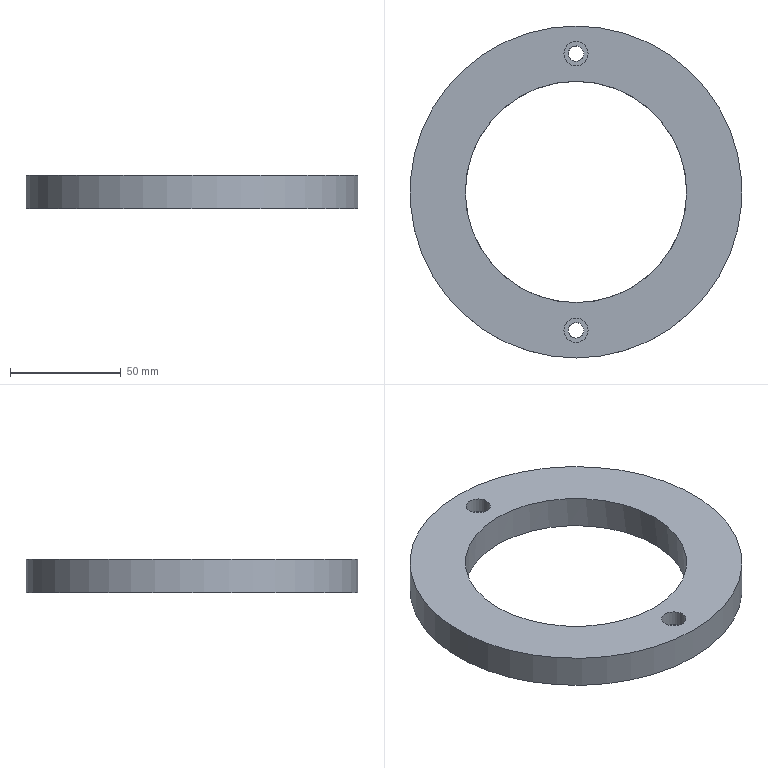Part | NX | features 模具.stp<1>[80] 2 | 1 solid | 10 faces | box 150 x 150 x 15 mm | volume 145316 mm3 | cylinder 6 | plane 4 | commonest cylinder face diameters 7 x2 11 x2 100 x1 150 x1
STEP:
#1=CARTESIAN_POINT('',(0.,-50.,150.5));
#2=VERTEX_POINT('',#1);
#3=CARTESIAN_POINT('',(0.,0.,150.5));
#4=DIRECTION('',(0.,0.,-1.));
#5=DIRECTION('',(0.,-1.,0.));
#6=AXIS2_PLACEMENT_3D('',#3,#4,#5);
#7=CIRCLE('',#6,50.);
#8=EDGE_CURVE('',#2,#2,#7,.T.);
#9=ORIENTED_EDGE('',*,*,#8,.F.);
#10=EDGE_LOOP('',(#9));
#11=FACE_BOUND('',#10,.T.);
#12=CARTESIAN_POINT('',(0.,50.,135.5));
#13=VERTEX_POINT('',#12);
#14=CARTESIAN_POINT('',(0.,0.,135.5));
#15=DIRECTION('',(0.,0.,1.));
#16=DIRECTION('',(0.,1.,0.));
#17=AXIS2_PLACEMENT_3D('',#14,#15,#16);
#18=CIRCLE('',#17,50.);
#19=EDGE_CURVE('',#13,#13,#18,.T.);
#20=ORIENTED_EDGE('',*,*,#19,.F.);
#21=EDGE_LOOP('',(#20));
#22=FACE_BOUND('',#21,.T.);
#23=CARTESIAN_POINT('',(0.,0.,150.5));
#24=DIRECTION('',(0.,0.,-1.));
#25=DIRECTION('',(0.,1.,0.));
#26=AXIS2_PLACEMENT_3D('',#23,#24,#25);
#27=CYLINDRICAL_SURFACE('',#26,50.);
#28=ADVANCED_FACE('',(#11,#22),#27,.F.);
#29=CARTESIAN_POINT('',(5.5,62.5,143.5));
#30=VERTEX_POINT('',#29);
#31=CARTESIAN_POINT('',(0.,62.5,143.5));
#32=DIRECTION('',(0.,0.,-1.));
#33=DIRECTION('',(1.,0.,0.));
#34=AXIS2_PLACEMENT_3D('',#31,#32,#33);
#35=CIRCLE('',#34,5.5);
#36=EDGE_CURVE('',#30,#30,#35,.T.);
#37=ORIENTED_EDGE('',*,*,#36,.T.);
#38=EDGE_LOOP('',(#37));
#39=FACE_BOUND('',#38,.T.);
#40=CARTESIAN_POINT('',(5.5,62.5,150.5));
#41=VERTEX_POINT('',#40);
#42=CARTESIAN_POINT('',(0.,62.5,150.5));
#43=DIRECTION('',(0.,0.,-1.));
#44=DIRECTION('',(1.,0.,0.));
#45=AXIS2_PLACEMENT_3D('',#42,#43,#44);
#46=CIRCLE('',#45,5.5);
#47=EDGE_CURVE('',#41,#41,#46,.T.);
#48=ORIENTED_EDGE('',*,*,#47,.F.);
#49=EDGE_LOOP('',(#48));
#50=FACE_BOUND('',#49,.T.);
#51=CARTESIAN_POINT('',(0.,62.5,143.5));
#52=DIRECTION('',(0.,0.,1.));
#53=DIRECTION('',(1.,0.,0.));
#54=AXIS2_PLACEMENT_3D('',#51,#52,#53);
#55=CYLINDRICAL_SURFACE('',#54,5.5);
#56=ADVANCED_FACE('',(#39,#50),#55,.F.);
#57=ORIENTED_EDGE('',*,*,#36,.F.);
#58=EDGE_LOOP('',(#57));
#59=FACE_BOUND('',#58,.T.);
#60=CARTESIAN_POINT('',(0.,59.,143.5));
#61=VERTEX_POINT('',#60);
#62=CARTESIAN_POINT('',(0.,62.5,143.5));
#63=DIRECTION('',(0.,0.,-1.));
#64=DIRECTION('',(0.,-1.,0.));
#65=AXIS2_PLACEMENT_3D('',#62,#63,#64);
#66=CIRCLE('',#65,3.5);
#67=EDGE_CURVE('',#61,#61,#66,.T.);
#68=ORIENTED_EDGE('',*,*,#67,.T.);
#69=EDGE_LOOP('',(#68));
#70=FACE_BOUND('',#69,.T.);
#71=CARTESIAN_POINT('',(0.,62.5,143.5));
#72=DIRECTION('',(0.,0.,-1.));
#73=DIRECTION('',(-1.,0.,0.));
#74=AXIS2_PLACEMENT_3D('',#71,#72,#73);
#75=PLANE('',#74);
#76=ADVANCED_FACE('',(#59,#70),#75,.F.);
#77=CARTESIAN_POINT('',(3.5,62.5,135.5));
#78=VERTEX_POINT('',#77);
#79=CARTESIAN_POINT('',(0.,62.5,135.5));
#80=DIRECTION('',(0.,0.,1.));
#81=DIRECTION('',(1.,0.,0.));
#82=AXIS2_PLACEMENT_3D('',#79,#80,#81);
#83=CIRCLE('',#82,3.5);
#84=EDGE_CURVE('',#78,#78,#83,.T.);
#85=ORIENTED_EDGE('',*,*,#84,.F.);
#86=EDGE_LOOP('',(#85));
#87=FACE_BOUND('',#86,.T.);
#88=ORIENTED_EDGE('',*,*,#67,.F.);
#89=EDGE_LOOP('',(#88));
#90=FACE_BOUND('',#89,.T.);
#91=CARTESIAN_POINT('',(0.,62.5,135.5));
#92=DIRECTION('',(0.,0.,1.));
#93=DIRECTION('',(1.,0.,0.));
#94=AXIS2_PLACEMENT_3D('',#91,#92,#93);
#95=CYLINDRICAL_SURFACE('',#94,3.5);
#96=ADVANCED_FACE('',(#87,#90),#95,.F.);
#97=CARTESIAN_POINT('',(5.5,-62.5,143.5));
#98=VERTEX_POINT('',#97);
#99=CARTESIAN_POINT('',(0.,-62.5,143.5));
#100=DIRECTION('',(0.,0.,-1.));
#101=DIRECTION('',(1.,0.,0.));
#102=AXIS2_PLACEMENT_3D('',#99,#100,#101);
#103=CIRCLE('',#102,5.5);
#104=EDGE_CURVE('',#98,#98,#103,.T.);
#105=ORIENTED_EDGE('',*,*,#104,.T.);
#106=EDGE_LOOP('',(#105));
#107=FACE_BOUND('',#106,.T.);
#108=CARTESIAN_POINT('',(5.5,-62.5,150.5));
#109=VERTEX_POINT('',#108);
#110=CARTESIAN_POINT('',(0.,-62.5,150.5));
#111=DIRECTION('',(0.,0.,-1.));
#112=DIRECTION('',(1.,0.,0.));
#113=AXIS2_PLACEMENT_3D('',#110,#111,#112);
#114=CIRCLE('',#113,5.5);
#115=EDGE_CURVE('',#109,#109,#114,.T.);
#116=ORIENTED_EDGE('',*,*,#115,.F.);
#117=EDGE_LOOP('',(#116));
#118=FACE_BOUND('',#117,.T.);
#119=CARTESIAN_POINT('',(0.,-62.5,143.5));
#120=DIRECTION('',(0.,0.,1.));
#121=DIRECTION('',(1.,0.,0.));
#122=AXIS2_PLACEMENT_3D('',#119,#120,#121);
#123=CYLINDRICAL_SURFACE('',#122,5.5);
#124=ADVANCED_FACE('',(#107,#118),#123,.F.);
#125=ORIENTED_EDGE('',*,*,#104,.F.);
#126=EDGE_LOOP('',(#125));
#127=FACE_BOUND('',#126,.T.);
#128=CARTESIAN_POINT('',(0.,-66.,143.5));
#129=VERTEX_POINT('',#128);
#130=CARTESIAN_POINT('',(0.,-62.5,143.5));
#131=DIRECTION('',(0.,0.,-1.));
#132=DIRECTION('',(0.,-1.,0.));
#133=AXIS2_PLACEMENT_3D('',#130,#131,#132);
#134=CIRCLE('',#133,3.5);
#135=EDGE_CURVE('',#129,#129,#134,.T.);
#136=ORIENTED_EDGE('',*,*,#135,.T.);
#137=EDGE_LOOP('',(#136));
#138=FACE_BOUND('',#137,.T.);
#139=CARTESIAN_POINT('',(0.,-62.5,143.5));
#140=DIRECTION('',(0.,0.,-1.));
#141=DIRECTION('',(-1.,0.,0.));
#142=AXIS2_PLACEMENT_3D('',#139,#140,#141);
#143=PLANE('',#142);
#144=ADVANCED_FACE('',(#127,#138),#143,.F.);
#145=CARTESIAN_POINT('',(3.5,-62.5,135.5));
#146=VERTEX_POINT('',#145);
#147=CARTESIAN_POINT('',(0.,-62.5,135.5));
#148=DIRECTION('',(0.,0.,1.));
#149=DIRECTION('',(1.,0.,0.));
#150=AXIS2_PLACEMENT_3D('',#147,#148,#149);
#151=CIRCLE('',#150,3.5);
#152=EDGE_CURVE('',#146,#146,#151,.T.);
#153=ORIENTED_EDGE('',*,*,#152,.F.);
#154=EDGE_LOOP('',(#153));
#155=FACE_BOUND('',#154,.T.);
#156=ORIENTED_EDGE('',*,*,#135,.F.);
#157=EDGE_LOOP('',(#156));
#158=FACE_BOUND('',#157,.T.);
#159=CARTESIAN_POINT('',(0.,-62.5,135.5));
#160=DIRECTION('',(0.,0.,1.));
#161=DIRECTION('',(1.,0.,0.));
#162=AXIS2_PLACEMENT_3D('',#159,#160,#161);
#163=CYLINDRICAL_SURFACE('',#162,3.5);
#164=ADVANCED_FACE('',(#155,#158),#163,.F.);
#165=CARTESIAN_POINT('',(0.,75.,135.5));
#166=VERTEX_POINT('',#165);
#167=CARTESIAN_POINT('',(0.,0.,135.5));
#168=DIRECTION('',(0.,0.,1.));
#169=DIRECTION('',(0.,1.,0.));
#170=AXIS2_PLACEMENT_3D('',#167,#168,#169);
#171=CIRCLE('',#170,75.);
#172=EDGE_CURVE('',#166,#166,#171,.T.);
#173=ORIENTED_EDGE('',*,*,#172,.T.);
#174=EDGE_LOOP('',(#173));
#175=FACE_BOUND('',#174,.T.);
#176=CARTESIAN_POINT('',(0.,-75.,150.5));
#177=VERTEX_POINT('',#176);
#178=CARTESIAN_POINT('',(0.,0.,150.5));
#179=DIRECTION('',(0.,0.,-1.));
#180=DIRECTION('',(0.,-1.,0.));
#181=AXIS2_PLACEMENT_3D('',#178,#179,#180);
#182=CIRCLE('',#181,75.);
#183=EDGE_CURVE('',#177,#177,#182,.T.);
#184=ORIENTED_EDGE('',*,*,#183,.T.);
#185=EDGE_LOOP('',(#184));
#186=FACE_BOUND('',#185,.T.);
#187=CARTESIAN_POINT('',(0.,0.,150.5));
#188=DIRECTION('',(0.,0.,-1.));
#189=DIRECTION('',(0.,1.,0.));
#190=AXIS2_PLACEMENT_3D('',#187,#188,#189);
#191=CYLINDRICAL_SURFACE('',#190,75.);
#192=ADVANCED_FACE('',(#175,#186),#191,.T.);
#193=ORIENTED_EDGE('',*,*,#8,.T.);
#194=EDGE_LOOP('',(#193));
#195=FACE_BOUND('',#194,.T.);
#196=ORIENTED_EDGE('',*,*,#183,.F.);
#197=EDGE_LOOP('',(#196));
#198=FACE_BOUND('',#197,.T.);
#199=ORIENTED_EDGE('',*,*,#47,.T.);
#200=EDGE_LOOP('',(#199));
#201=FACE_BOUND('',#200,.T.);
#202=ORIENTED_EDGE('',*,*,#115,.T.);
#203=EDGE_LOOP('',(#202));
#204=FACE_BOUND('',#203,.T.);
#205=CARTESIAN_POINT('',(0.,0.,150.5));
#206=DIRECTION('',(0.,0.,1.));
#207=DIRECTION('',(0.,-1.,0.));
#208=AXIS2_PLACEMENT_3D('',#205,#206,#207);
#209=PLANE('',#208);
#210=ADVANCED_FACE('',(#195,#198,#201,#204),#209,.T.);
#211=ORIENTED_EDGE('',*,*,#19,.T.);
#212=EDGE_LOOP('',(#211));
#213=FACE_BOUND('',#212,.T.);
#214=ORIENTED_EDGE('',*,*,#172,.F.);
#215=EDGE_LOOP('',(#214));
#216=FACE_BOUND('',#215,.T.);
#217=ORIENTED_EDGE('',*,*,#84,.T.);
#218=EDGE_LOOP('',(#217));
#219=FACE_BOUND('',#218,.T.);
#220=ORIENTED_EDGE('',*,*,#152,.T.);
#221=EDGE_LOOP('',(#220));
#222=FACE_BOUND('',#221,.T.);
#223=CARTESIAN_POINT('',(0.,0.,135.5));
#224=DIRECTION('',(0.,0.,-1.));
#225=DIRECTION('',(-1.,0.,0.));
#226=AXIS2_PLACEMENT_3D('',#223,#224,#225);
#227=PLANE('',#226);
#228=ADVANCED_FACE('',(#213,#216,#219,#222),#227,.T.);
#229=CLOSED_SHELL('',(#28,#56,#76,#96,#124,#144,#164,#192,#210,#228));
#230=MANIFOLD_SOLID_BREP('',#229);
#231=(LENGTH_UNIT()NAMED_UNIT(*)SI_UNIT(.MILLI.,.METRE.));
#232=UNCERTAINTY_MEASURE_WITH_UNIT(LENGTH_MEASURE(0.00001),#231,'','');
#233=(NAMED_UNIT(*)PLANE_ANGLE_UNIT()SI_UNIT($,.RADIAN.));
#234=(NAMED_UNIT(*)SI_UNIT($,.STERADIAN.)SOLID_ANGLE_UNIT());
#235=(GEOMETRIC_REPRESENTATION_CONTEXT(3)GLOBAL_UNCERTAINTY_ASSIGNED_CONTEXT((#232))GLOBAL_UNIT_ASSIGNED_CONTEXT((#231,#233,#234))REPRESENTATION_CONTEXT('',''));
#236=ADVANCED_BREP_SHAPE_REPRESENTATION('',(#230),#235);